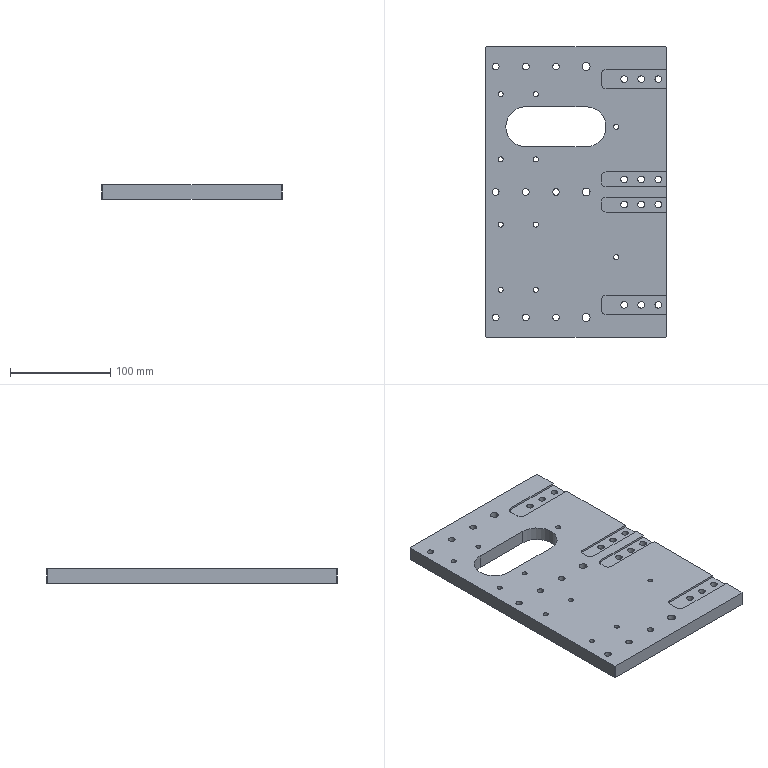Part | NX | features BREP 1 | 1 solid | 170 faces | box 180 x 290 x 14 mm | volume 649095 mm3 | cylinder 121 | plane 49 | commonest cylinder face diameters 10 x26 6.6 x24 11 x24 5 x20 6.5 x18 8 x6